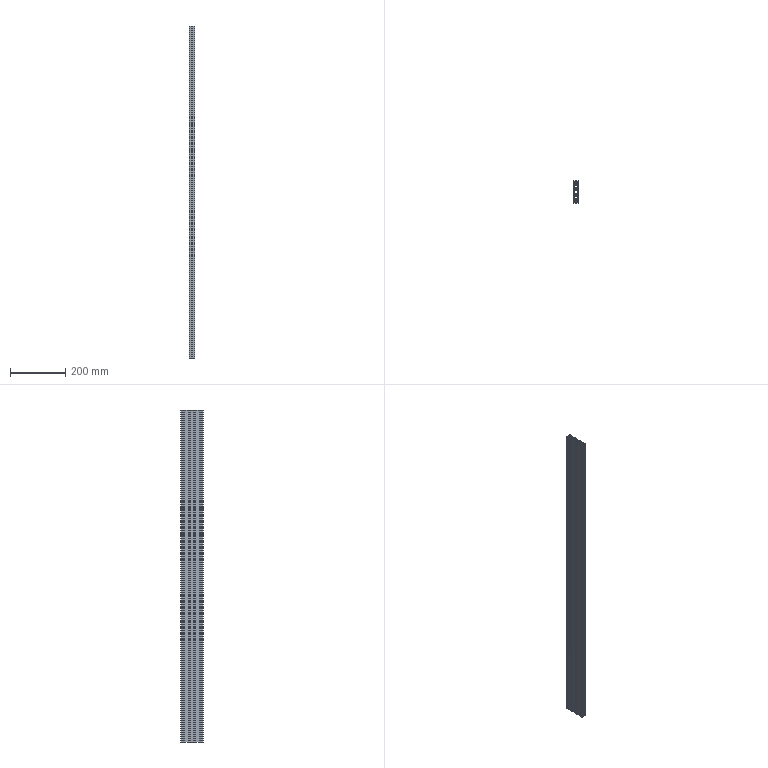Part | STEP file | HFS5-2080-1198_HFS5-2080-1380 | 1 solid | 204 faces | box 20 x 80 x 1198 mm | volume 727217 mm3 | plane 172 | cylinder 32 | commonest cylinder face diameters 0.6 x20 4.2 x8 2 x4